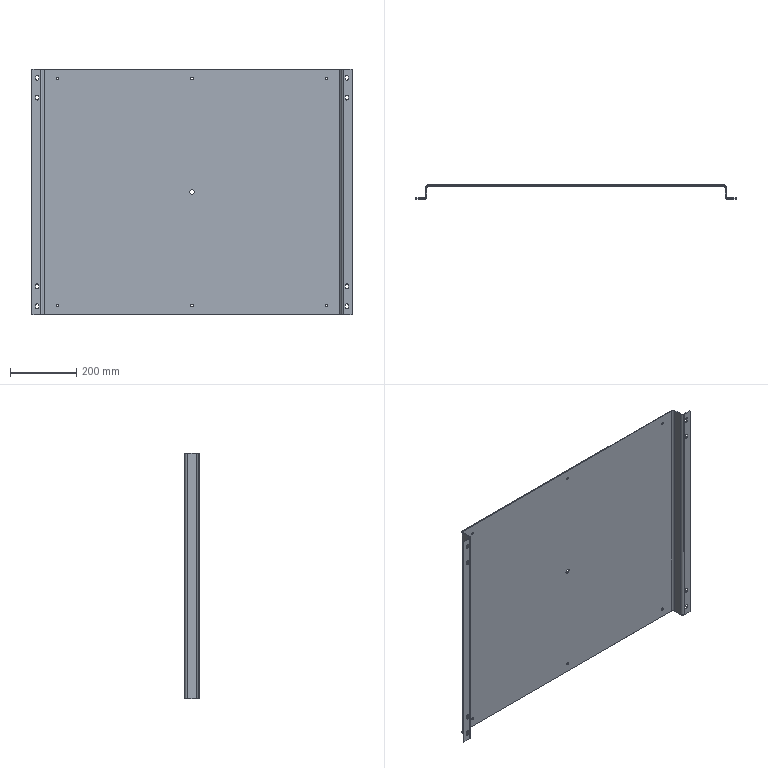Part | SolidWorks | features ICE 3, Extrusion 1 | 1 solid | 76 faces | box 966 x 43 x 740 mm | volume 2293433 mm3 | cylinder 46 | plane 30 | commonest cylinder face diameters 9 x24 7 x12 10 x4 16 x4 13 x2